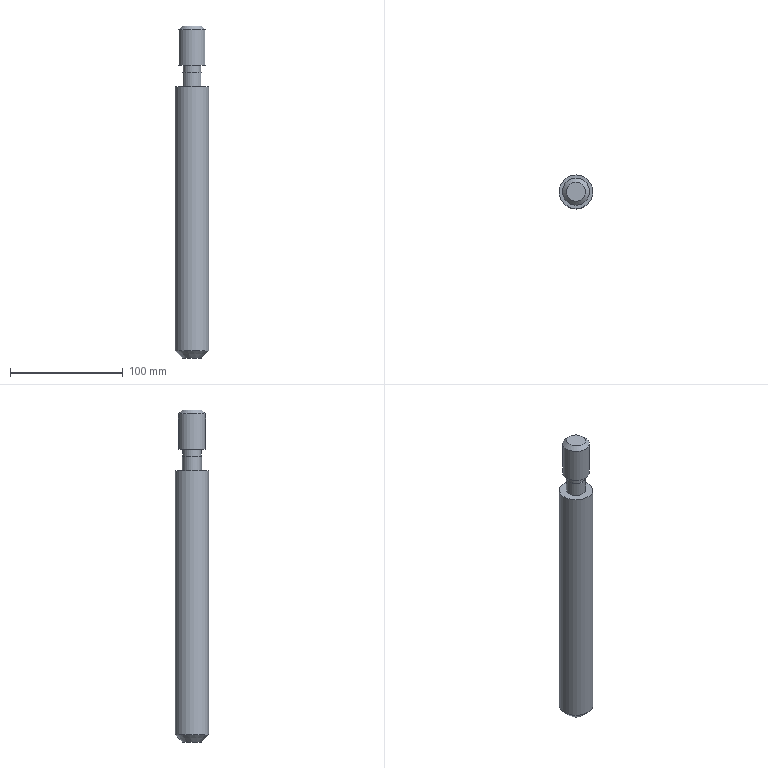Part | NX | features solid 2 | 1 solid | 11 faces | box 30 x 30 x 295 mm | volume 188223 mm3 | plane 5 | cylinder 4 | cone 2 | commonest cylinder face diameters 16 x1 17 x1 24 x1 30 x1
STEP:
#1=CARTESIAN_POINT('',(209.887,-11.281,-159.));
#2=VERTEX_POINT('',#1);
#3=CARTESIAN_POINT('',(209.887,-11.281,-149.));
#4=VERTEX_POINT('',#3);
#5=CARTESIAN_POINT('',(209.887,-11.281,-382.));
#6=DIRECTION('',(0.,0.,1.));
#7=VECTOR('',#6,1000.);
#8=LINE('',#5,#7);
#9=EDGE_CURVE('',#2,#4,#8,.T.);
#10=ORIENTED_EDGE('',*,*,#9,.F.);
#11=ORIENTED_EDGE('',*,*,#9,.T.);
#12=EDGE_LOOP('',(#10,#11));
#13=FACE_BOUND('',#12,.T.);
#14=CARTESIAN_POINT('',(200.,-15.,-375.5));
#15=VERTEX_POINT('',#14);
#16=CARTESIAN_POINT('',(200.,0.,-375.5));
#17=DIRECTION('',(0.,0.,1.));
#18=DIRECTION('',(0.,-1.,0.));
#19=AXIS2_PLACEMENT_3D('',#16,#17,#18);
#20=CIRCLE('',#19,15.);
#21=EDGE_CURVE('',#15,#15,#20,.T.);
#22=ORIENTED_EDGE('',*,*,#21,.T.);
#23=EDGE_LOOP('',(#22));
#24=FACE_BOUND('',#23,.T.);
#25=CARTESIAN_POINT('',(200.,15.,-141.));
#26=VERTEX_POINT('',#25);
#27=CARTESIAN_POINT('',(200.,0.,-141.));
#28=DIRECTION('',(0.,0.,-1.));
#29=DIRECTION('',(0.,1.,0.));
#30=AXIS2_PLACEMENT_3D('',#27,#28,#29);
#31=CIRCLE('',#30,15.);
#32=EDGE_CURVE('',#26,#26,#31,.F.);
#33=ORIENTED_EDGE('',*,*,#32,.F.);
#34=EDGE_LOOP('',(#33));
#35=FACE_BOUND('',#34,.T.);
#36=CARTESIAN_POINT('',(190.113,-11.281,-159.));
#37=VERTEX_POINT('',#36);
#38=CARTESIAN_POINT('',(190.113,-11.281,-149.));
#39=VERTEX_POINT('',#38);
#40=CARTESIAN_POINT('',(190.113,-11.281,-382.));
#41=DIRECTION('',(0.,0.,1.));
#42=VECTOR('',#41,1000.);
#43=LINE('',#40,#42);
#44=EDGE_CURVE('',#37,#39,#43,.T.);
#45=ORIENTED_EDGE('',*,*,#44,.F.);
#46=ORIENTED_EDGE('',*,*,#44,.T.);
#47=EDGE_LOOP('',(#45,#46));
#48=FACE_BOUND('',#47,.T.);
#49=CARTESIAN_POINT('',(200.,0.,-382.));
#50=DIRECTION('',(0.,0.,1.));
#51=DIRECTION('',(0.,1.,0.));
#52=AXIS2_PLACEMENT_3D('',#49,#50,#51);
#53=CYLINDRICAL_SURFACE('',#52,15.);
#54=ADVANCED_FACE('',(#13,#24,#35,#48),#53,.T.);
#55=CARTESIAN_POINT('',(200.,8.5,-382.));
#56=VERTEX_POINT('',#55);
#57=CARTESIAN_POINT('',(200.,0.,-382.));
#58=DIRECTION('',(0.,0.,-1.));
#59=DIRECTION('',(0.,1.,0.));
#60=AXIS2_PLACEMENT_3D('',#57,#58,#59);
#61=CIRCLE('',#60,8.5);
#62=EDGE_CURVE('',#56,#56,#61,.T.);
#63=ORIENTED_EDGE('',*,*,#62,.T.);
#64=EDGE_LOOP('',(#63));
#65=FACE_BOUND('',#64,.T.);
#66=CARTESIAN_POINT('',(200.,0.,-382.));
#67=DIRECTION('',(0.,0.,-1.));
#68=DIRECTION('',(0.,-1.,0.));
#69=AXIS2_PLACEMENT_3D('',#66,#67,#68);
#70=PLANE('',#69);
#71=ADVANCED_FACE('',(#65),#70,.T.);
#72=CARTESIAN_POINT('',(200.,8.5,-128.));
#73=VERTEX_POINT('',#72);
#74=CARTESIAN_POINT('',(200.,0.,-128.));
#75=DIRECTION('',(0.,0.,-1.));
#76=DIRECTION('',(0.,1.,0.));
#77=AXIS2_PLACEMENT_3D('',#74,#75,#76);
#78=CIRCLE('',#77,8.5);
#79=EDGE_CURVE('',#73,#73,#78,.T.);
#80=ORIENTED_EDGE('',*,*,#79,.T.);
#81=EDGE_LOOP('',(#80));
#82=FACE_BOUND('',#81,.T.);
#83=CARTESIAN_POINT('',(200.,8.5,-141.));
#84=VERTEX_POINT('',#83);
#85=CARTESIAN_POINT('',(200.,0.,-141.));
#86=DIRECTION('',(0.,0.,1.));
#87=DIRECTION('',(0.,1.,0.));
#88=AXIS2_PLACEMENT_3D('',#85,#86,#87);
#89=CIRCLE('',#88,8.5);
#90=EDGE_CURVE('',#84,#84,#89,.T.);
#91=ORIENTED_EDGE('',*,*,#90,.T.);
#92=EDGE_LOOP('',(#91));
#93=FACE_BOUND('',#92,.T.);
#94=CARTESIAN_POINT('',(200.,0.,-141.));
#95=DIRECTION('',(0.,0.,1.));
#96=DIRECTION('',(0.,1.,0.));
#97=AXIS2_PLACEMENT_3D('',#94,#95,#96);
#98=CYLINDRICAL_SURFACE('',#97,8.5);
#99=ADVANCED_FACE('',(#82,#93),#98,.T.);
#100=ORIENTED_EDGE('',*,*,#90,.F.);
#101=EDGE_LOOP('',(#100));
#102=FACE_BOUND('',#101,.T.);
#103=ORIENTED_EDGE('',*,*,#32,.T.);
#104=EDGE_LOOP('',(#103));
#105=FACE_BOUND('',#104,.T.);
#106=CARTESIAN_POINT('',(200.,0.,-141.));
#107=DIRECTION('',(0.,0.,-1.));
#108=DIRECTION('',(0.,-1.,0.));
#109=AXIS2_PLACEMENT_3D('',#106,#107,#108);
#110=PLANE('',#109);
#111=ADVANCED_FACE('',(#102,#105),#110,.F.);
#112=CARTESIAN_POINT('',(200.,8.,-128.));
#113=VERTEX_POINT('',#112);
#114=CARTESIAN_POINT('',(200.,0.,-128.));
#115=DIRECTION('',(0.,0.,1.));
#116=DIRECTION('',(0.,1.,0.));
#117=AXIS2_PLACEMENT_3D('',#114,#115,#116);
#118=CIRCLE('',#117,8.);
#119=EDGE_CURVE('',#113,#113,#118,.T.);
#120=ORIENTED_EDGE('',*,*,#119,.F.);
#121=EDGE_LOOP('',(#120));
#122=FACE_BOUND('',#121,.T.);
#123=ORIENTED_EDGE('',*,*,#79,.F.);
#124=EDGE_LOOP('',(#123));
#125=FACE_BOUND('',#124,.T.);
#126=CARTESIAN_POINT('',(200.,0.,-128.));
#127=DIRECTION('',(0.,0.,-1.));
#128=DIRECTION('',(0.,-1.,0.));
#129=AXIS2_PLACEMENT_3D('',#126,#127,#128);
#130=PLANE('',#129);
#131=ADVANCED_FACE('',(#122,#125),#130,.F.);
#132=ORIENTED_EDGE('',*,*,#119,.T.);
#133=EDGE_LOOP('',(#132));
#134=FACE_BOUND('',#133,.T.);
#135=CARTESIAN_POINT('',(200.,8.,-122.));
#136=VERTEX_POINT('',#135);
#137=CARTESIAN_POINT('',(200.,0.,-122.));
#138=DIRECTION('',(0.,0.,1.));
#139=DIRECTION('',(0.,1.,0.));
#140=AXIS2_PLACEMENT_3D('',#137,#138,#139);
#141=CIRCLE('',#140,8.);
#142=EDGE_CURVE('',#136,#136,#141,.T.);
#143=ORIENTED_EDGE('',*,*,#142,.F.);
#144=EDGE_LOOP('',(#143));
#145=FACE_BOUND('',#144,.T.);
#146=CARTESIAN_POINT('',(200.,0.,-128.));
#147=DIRECTION('',(0.,0.,1.));
#148=DIRECTION('',(0.,1.,0.));
#149=AXIS2_PLACEMENT_3D('',#146,#147,#148);
#150=CYLINDRICAL_SURFACE('',#149,8.);
#151=ADVANCED_FACE('',(#134,#145),#150,.T.);
#152=CARTESIAN_POINT('',(200.,8.5,-87.));
#153=VERTEX_POINT('',#152);
#154=CARTESIAN_POINT('',(200.,0.,-87.));
#155=DIRECTION('',(0.,0.,-1.));
#156=DIRECTION('',(0.,1.,0.));
#157=AXIS2_PLACEMENT_3D('',#154,#155,#156);
#158=CIRCLE('',#157,8.5);
#159=EDGE_CURVE('',#153,#153,#158,.F.);
#160=ORIENTED_EDGE('',*,*,#159,.T.);
#161=EDGE_LOOP('',(#160));
#162=FACE_BOUND('',#161,.T.);
#163=CARTESIAN_POINT('',(200.,0.,-87.));
#164=DIRECTION('',(0.,0.,-1.));
#165=DIRECTION('',(0.,-1.,0.));
#166=AXIS2_PLACEMENT_3D('',#163,#164,#165);
#167=PLANE('',#166);
#168=ADVANCED_FACE('',(#162),#167,.F.);
#169=CARTESIAN_POINT('',(200.,12.,-90.5));
#170=VERTEX_POINT('',#169);
#171=CARTESIAN_POINT('',(200.,0.,-90.5));
#172=DIRECTION('',(0.,0.,-1.));
#173=DIRECTION('',(0.,1.,0.));
#174=AXIS2_PLACEMENT_3D('',#171,#172,#173);
#175=CIRCLE('',#174,12.);
#176=EDGE_CURVE('',#170,#170,#175,.T.);
#177=ORIENTED_EDGE('',*,*,#176,.T.);
#178=EDGE_LOOP('',(#177));
#179=FACE_BOUND('',#178,.T.);
#180=CARTESIAN_POINT('',(200.,12.,-122.));
#181=VERTEX_POINT('',#180);
#182=CARTESIAN_POINT('',(200.,0.,-122.));
#183=DIRECTION('',(0.,0.,-1.));
#184=DIRECTION('',(0.,1.,0.));
#185=AXIS2_PLACEMENT_3D('',#182,#183,#184);
#186=CIRCLE('',#185,12.);
#187=EDGE_CURVE('',#181,#181,#186,.F.);
#188=ORIENTED_EDGE('',*,*,#187,.T.);
#189=EDGE_LOOP('',(#188));
#190=FACE_BOUND('',#189,.T.);
#191=CARTESIAN_POINT('',(200.,0.,-382.));
#192=DIRECTION('',(0.,0.,1.));
#193=DIRECTION('',(0.,1.,0.));
#194=AXIS2_PLACEMENT_3D('',#191,#192,#193);
#195=CYLINDRICAL_SURFACE('',#194,12.);
#196=ADVANCED_FACE('',(#179,#190),#195,.T.);
#197=ORIENTED_EDGE('',*,*,#187,.F.);
#198=EDGE_LOOP('',(#197));
#199=FACE_BOUND('',#198,.T.);
#200=ORIENTED_EDGE('',*,*,#142,.T.);
#201=EDGE_LOOP('',(#200));
#202=FACE_BOUND('',#201,.T.);
#203=CARTESIAN_POINT('',(200.,0.,-122.));
#204=DIRECTION('',(0.,0.,-1.));
#205=DIRECTION('',(0.,-1.,0.));
#206=AXIS2_PLACEMENT_3D('',#203,#204,#205);
#207=PLANE('',#206);
#208=ADVANCED_FACE('',(#199,#202),#207,.T.);
#209=ORIENTED_EDGE('',*,*,#62,.F.);
#210=EDGE_LOOP('',(#209));
#211=FACE_BOUND('',#210,.T.);
#212=ORIENTED_EDGE('',*,*,#21,.F.);
#213=EDGE_LOOP('',(#212));
#214=FACE_BOUND('',#213,.T.);
#215=CARTESIAN_POINT('',(200.,0.,-381.5));
#216=DIRECTION('',(0.,0.,1.));
#217=DIRECTION('',(0.,-1.,0.));
#218=AXIS2_PLACEMENT_3D('',#215,#216,#217);
#219=CONICAL_SURFACE('',#218,9.,0.7854);
#220=ADVANCED_FACE('',(#211,#214),#219,.T.);
#221=ORIENTED_EDGE('',*,*,#176,.F.);
#222=EDGE_LOOP('',(#221));
#223=FACE_BOUND('',#222,.T.);
#224=ORIENTED_EDGE('',*,*,#159,.F.);
#225=EDGE_LOOP('',(#224));
#226=FACE_BOUND('',#225,.T.);
#227=CARTESIAN_POINT('',(200.,0.,-87.));
#228=DIRECTION('',(0.,0.,-1.));
#229=DIRECTION('',(0.,1.,0.));
#230=AXIS2_PLACEMENT_3D('',#227,#228,#229);
#231=CONICAL_SURFACE('',#230,8.5,0.7854);
#232=ADVANCED_FACE('',(#223,#226),#231,.T.);
#233=CLOSED_SHELL('',(#54,#71,#99,#111,#131,#151,#168,#196,#208,#220,#232));
#234=MANIFOLD_SOLID_BREP('',#233);
#235=(LENGTH_UNIT()NAMED_UNIT(*)SI_UNIT(.MILLI.,.METRE.));
#236=UNCERTAINTY_MEASURE_WITH_UNIT(LENGTH_MEASURE(0.00001),#235,'','');
#237=(NAMED_UNIT(*)PLANE_ANGLE_UNIT()SI_UNIT($,.RADIAN.));
#238=(NAMED_UNIT(*)SI_UNIT($,.STERADIAN.)SOLID_ANGLE_UNIT());
#239=(GEOMETRIC_REPRESENTATION_CONTEXT(3)GLOBAL_UNCERTAINTY_ASSIGNED_CONTEXT((#236))GLOBAL_UNIT_ASSIGNED_CONTEXT((#235,#237,#238))REPRESENTATION_CONTEXT('',''));
#240=ADVANCED_BREP_SHAPE_REPRESENTATION('',(#234),#239);